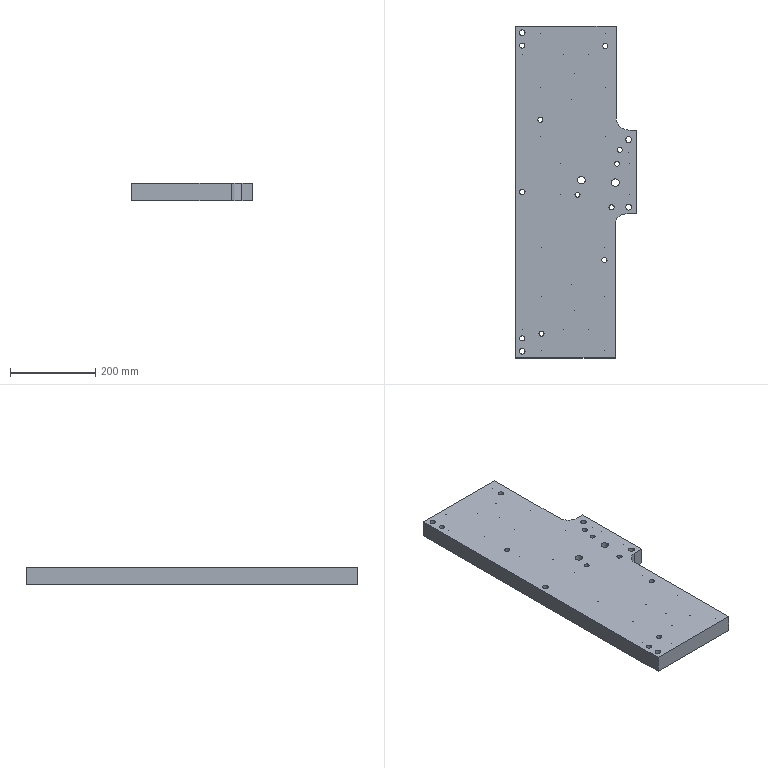Part | STEP file | lll_id2978_x_t | 1 solid | 93 faces | box 285 x 780 x 40 mm | volume 7562458 mm3 | cylinder 51 | cone 27 | plane 15 | commonest cylinder face diameters 10.506 x24 12 x10 13.509 x5 20.007 x5 10.505 x3 18 x2